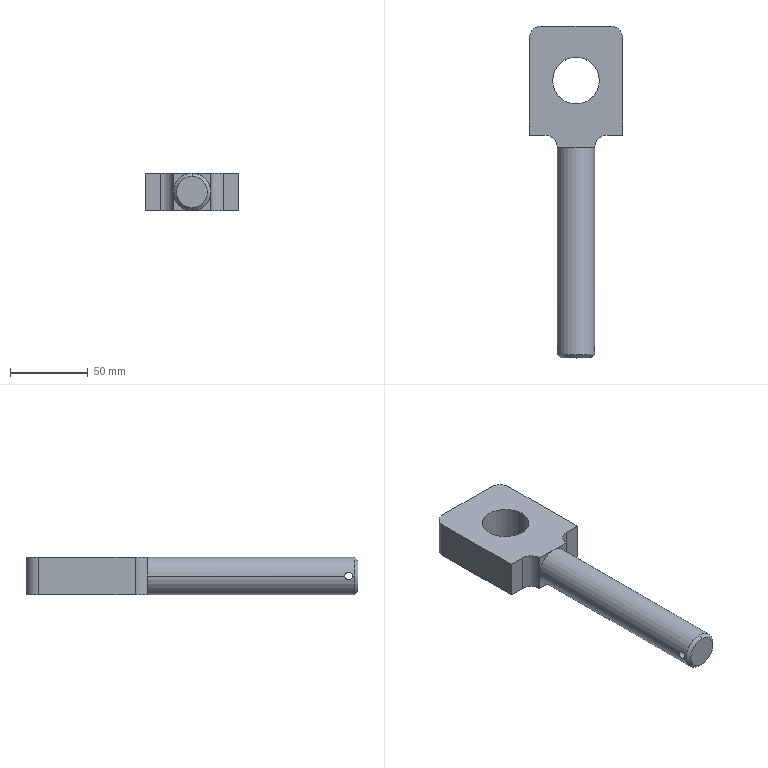Part | STEP file | Lifting fork tie rod | 1 solid | 24 faces | box 60 x 213 x 24 mm | volume 148905 mm3 | plane 12 | cylinder 10 | cone 2 | commonest cylinder face diameters 16 x4 5 x2 24 x2 30 x2